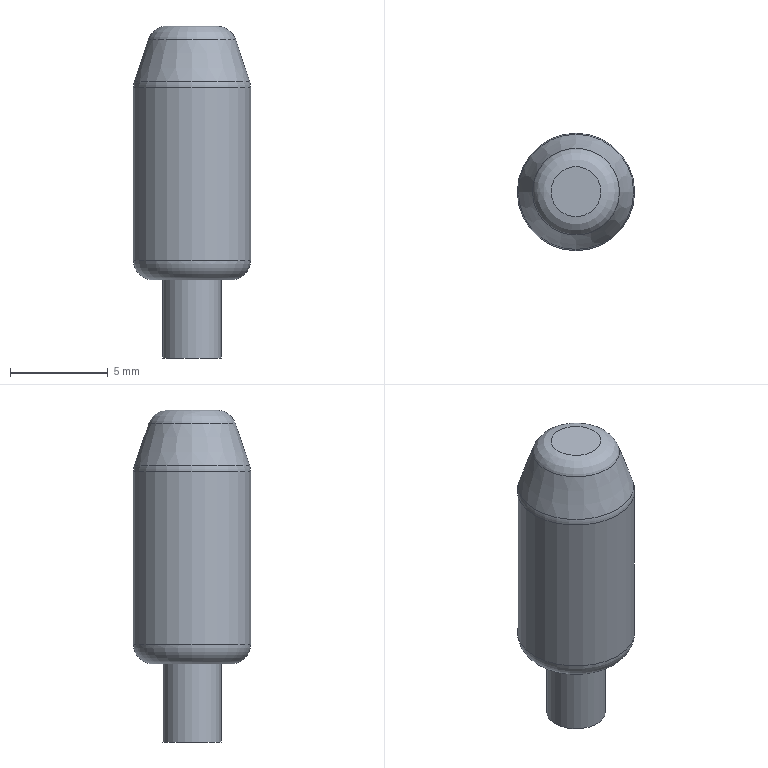Part | NX | features DATUM_CSYS 2, BLEND 1, SKETCH 1, SWP104 1 | 1 solid | 9 faces | box 6 x 6 x 17 mm | volume 365.792 mm3 | plane 3 | torus 3 | cylinder 2 | cone 1 | commonest cylinder face diameters 3 x1 6 x1
STEP:
#1=CARTESIAN_POINT('',(3.,0.,1.));
#2=VERTEX_POINT('',#1);
#3=CARTESIAN_POINT('',(0.,0.,1.));
#4=DIRECTION('',(0.,0.,1.));
#5=DIRECTION('',(1.,0.,0.));
#6=AXIS2_PLACEMENT_3D('',#3,#4,#5);
#7=CIRCLE('',#6,3.);
#8=EDGE_CURVE('',#2,#2,#7,.T.);
#9=ORIENTED_EDGE('',*,*,#8,.T.);
#10=EDGE_LOOP('',(#9));
#11=FACE_BOUND('',#10,.T.);
#12=CARTESIAN_POINT('',(3.,0.,9.838));
#13=VERTEX_POINT('',#12);
#14=CARTESIAN_POINT('',(0.,0.,9.838));
#15=DIRECTION('',(0.,0.,1.));
#16=DIRECTION('',(1.,0.,0.));
#17=AXIS2_PLACEMENT_3D('',#14,#15,#16);
#18=CIRCLE('',#17,3.);
#19=EDGE_CURVE('',#13,#13,#18,.F.);
#20=ORIENTED_EDGE('',*,*,#19,.T.);
#21=EDGE_LOOP('',(#20));
#22=FACE_BOUND('',#21,.T.);
#23=CARTESIAN_POINT('',(0.,0.,0.));
#24=DIRECTION('',(0.,0.,-1.));
#25=DIRECTION('',(-1.,0.,0.));
#26=AXIS2_PLACEMENT_3D('',#23,#24,#25);
#27=CYLINDRICAL_SURFACE('',#26,3.);
#28=ADVANCED_FACE('',(#11,#22),#27,.T.);
#29=CARTESIAN_POINT('',(2.,0.,0.));
#30=VERTEX_POINT('',#29);
#31=CARTESIAN_POINT('',(0.,0.,0.));
#32=DIRECTION('',(0.,0.,1.));
#33=DIRECTION('',(1.,0.,0.));
#34=AXIS2_PLACEMENT_3D('',#31,#32,#33);
#35=CIRCLE('',#34,2.);
#36=EDGE_CURVE('',#30,#30,#35,.F.);
#37=ORIENTED_EDGE('',*,*,#36,.T.);
#38=EDGE_LOOP('',(#37));
#39=FACE_BOUND('',#38,.T.);
#40=CARTESIAN_POINT('',(-1.5,0.,0.));
#41=VERTEX_POINT('',#40);
#42=CARTESIAN_POINT('',(0.,0.,0.));
#43=DIRECTION('',(0.,0.,-1.));
#44=DIRECTION('',(-1.,0.,0.));
#45=AXIS2_PLACEMENT_3D('',#42,#43,#44);
#46=CIRCLE('',#45,1.5);
#47=EDGE_CURVE('',#41,#41,#46,.T.);
#48=ORIENTED_EDGE('',*,*,#47,.F.);
#49=EDGE_LOOP('',(#48));
#50=FACE_BOUND('',#49,.T.);
#51=CARTESIAN_POINT('',(0.,-3.,0.));
#52=DIRECTION('',(0.,0.,1.));
#53=DIRECTION('',(1.,0.,0.));
#54=AXIS2_PLACEMENT_3D('',#51,#52,#53);
#55=PLANE('',#54);
#56=ADVANCED_FACE('',(#39,#50),#55,.F.);
#57=CARTESIAN_POINT('',(-1.5,0.,-4.));
#58=VERTEX_POINT('',#57);
#59=CARTESIAN_POINT('',(0.,0.,-4.));
#60=DIRECTION('',(0.,0.,-1.));
#61=DIRECTION('',(-1.,0.,0.));
#62=AXIS2_PLACEMENT_3D('',#59,#60,#61);
#63=CIRCLE('',#62,1.5);
#64=EDGE_CURVE('',#58,#58,#63,.T.);
#65=ORIENTED_EDGE('',*,*,#64,.F.);
#66=EDGE_LOOP('',(#65));
#67=FACE_BOUND('',#66,.T.);
#68=ORIENTED_EDGE('',*,*,#47,.T.);
#69=EDGE_LOOP('',(#68));
#70=FACE_BOUND('',#69,.T.);
#71=CARTESIAN_POINT('',(0.,0.,0.));
#72=DIRECTION('',(0.,0.,-1.));
#73=DIRECTION('',(-1.,0.,0.));
#74=AXIS2_PLACEMENT_3D('',#71,#72,#73);
#75=CYLINDRICAL_SURFACE('',#74,1.5);
#76=ADVANCED_FACE('',(#67,#70),#75,.T.);
#77=ORIENTED_EDGE('',*,*,#64,.T.);
#78=EDGE_LOOP('',(#77));
#79=FACE_BOUND('',#78,.T.);
#80=CARTESIAN_POINT('',(0.,-1.5,-4.));
#81=DIRECTION('',(0.,0.,1.));
#82=DIRECTION('',(1.,0.,0.));
#83=AXIS2_PLACEMENT_3D('',#80,#81,#82);
#84=PLANE('',#83);
#85=ADVANCED_FACE('',(#79),#84,.F.);
#86=CARTESIAN_POINT('',(-1.279,0.,13.));
#87=VERTEX_POINT('',#86);
#88=CARTESIAN_POINT('',(0.,0.,13.));
#89=DIRECTION('',(0.,0.,-1.));
#90=DIRECTION('',(-1.,0.,0.));
#91=AXIS2_PLACEMENT_3D('',#88,#89,#90);
#92=CIRCLE('',#91,1.279);
#93=EDGE_CURVE('',#87,#87,#92,.F.);
#94=ORIENTED_EDGE('',*,*,#93,.T.);
#95=EDGE_LOOP('',(#94));
#96=FACE_BOUND('',#95,.T.);
#97=CARTESIAN_POINT('',(0.,0.,13.));
#98=DIRECTION('',(0.,0.,-1.));
#99=DIRECTION('',(-1.,0.,0.));
#100=AXIS2_PLACEMENT_3D('',#97,#98,#99);
#101=PLANE('',#100);
#102=ADVANCED_FACE('',(#96),#101,.F.);
#103=CARTESIAN_POINT('',(2.949,0.,10.154));
#104=VERTEX_POINT('',#103);
#105=CARTESIAN_POINT('',(0.,0.,10.154));
#106=DIRECTION('',(0.,0.,1.));
#107=DIRECTION('',(1.,0.,0.));
#108=AXIS2_PLACEMENT_3D('',#105,#106,#107);
#109=CIRCLE('',#108,2.949);
#110=EDGE_CURVE('',#104,#104,#109,.T.);
#111=ORIENTED_EDGE('',*,*,#110,.T.);
#112=EDGE_LOOP('',(#111));
#113=FACE_BOUND('',#112,.T.);
#114=CARTESIAN_POINT('',(2.228,0.,12.316));
#115=VERTEX_POINT('',#114);
#116=CARTESIAN_POINT('',(0.,0.,12.316));
#117=DIRECTION('',(0.,0.,1.));
#118=DIRECTION('',(1.,0.,0.));
#119=AXIS2_PLACEMENT_3D('',#116,#117,#118);
#120=CIRCLE('',#119,2.228);
#121=EDGE_CURVE('',#115,#115,#120,.F.);
#122=ORIENTED_EDGE('',*,*,#121,.T.);
#123=EDGE_LOOP('',(#122));
#124=FACE_BOUND('',#123,.T.);
#125=CARTESIAN_POINT('',(0.,0.,13.));
#126=DIRECTION('',(0.,0.,-1.));
#127=DIRECTION('',(-1.,0.,0.));
#128=AXIS2_PLACEMENT_3D('',#125,#126,#127);
#129=CONICAL_SURFACE('',#128,2.,0.3218);
#130=ADVANCED_FACE('',(#113,#124),#129,.T.);
#131=ORIENTED_EDGE('',*,*,#8,.F.);
#132=EDGE_LOOP('',(#131));
#133=FACE_BOUND('',#132,.T.);
#134=ORIENTED_EDGE('',*,*,#36,.F.);
#135=EDGE_LOOP('',(#134));
#136=FACE_BOUND('',#135,.T.);
#137=CARTESIAN_POINT('',(0.,0.,1.));
#138=DIRECTION('',(0.,0.,1.));
#139=DIRECTION('',(1.,0.,0.));
#140=AXIS2_PLACEMENT_3D('',#137,#138,#139);
#141=TOROIDAL_SURFACE('',#140,2.,1.);
#142=ADVANCED_FACE('',(#133,#136),#141,.T.);
#143=ORIENTED_EDGE('',*,*,#110,.F.);
#144=EDGE_LOOP('',(#143));
#145=FACE_BOUND('',#144,.T.);
#146=ORIENTED_EDGE('',*,*,#19,.F.);
#147=EDGE_LOOP('',(#146));
#148=FACE_BOUND('',#147,.T.);
#149=CARTESIAN_POINT('',(0.,0.,9.838));
#150=DIRECTION('',(0.,0.,1.));
#151=DIRECTION('',(1.,0.,0.));
#152=AXIS2_PLACEMENT_3D('',#149,#150,#151);
#153=TOROIDAL_SURFACE('',#152,2.,1.);
#154=ADVANCED_FACE('',(#145,#148),#153,.T.);
#155=ORIENTED_EDGE('',*,*,#93,.F.);
#156=EDGE_LOOP('',(#155));
#157=FACE_BOUND('',#156,.T.);
#158=ORIENTED_EDGE('',*,*,#121,.F.);
#159=EDGE_LOOP('',(#158));
#160=FACE_BOUND('',#159,.T.);
#161=CARTESIAN_POINT('',(0.,0.,12.));
#162=DIRECTION('',(0.,0.,-1.));
#163=DIRECTION('',(-1.,0.,0.));
#164=AXIS2_PLACEMENT_3D('',#161,#162,#163);
#165=TOROIDAL_SURFACE('',#164,1.279,1.);
#166=ADVANCED_FACE('',(#157,#160),#165,.T.);
#167=CLOSED_SHELL('',(#28,#56,#76,#85,#102,#130,#142,#154,#166));
#168=MANIFOLD_SOLID_BREP('',#167);
#169=(LENGTH_UNIT()NAMED_UNIT(*)SI_UNIT(.MILLI.,.METRE.));
#170=UNCERTAINTY_MEASURE_WITH_UNIT(LENGTH_MEASURE(0.00001),#169,'','');
#171=(NAMED_UNIT(*)PLANE_ANGLE_UNIT()SI_UNIT($,.RADIAN.));
#172=(NAMED_UNIT(*)SI_UNIT($,.STERADIAN.)SOLID_ANGLE_UNIT());
#173=(GEOMETRIC_REPRESENTATION_CONTEXT(3)GLOBAL_UNCERTAINTY_ASSIGNED_CONTEXT((#170))GLOBAL_UNIT_ASSIGNED_CONTEXT((#169,#171,#172))REPRESENTATION_CONTEXT('',''));
#174=ADVANCED_BREP_SHAPE_REPRESENTATION('',(#168),#173);